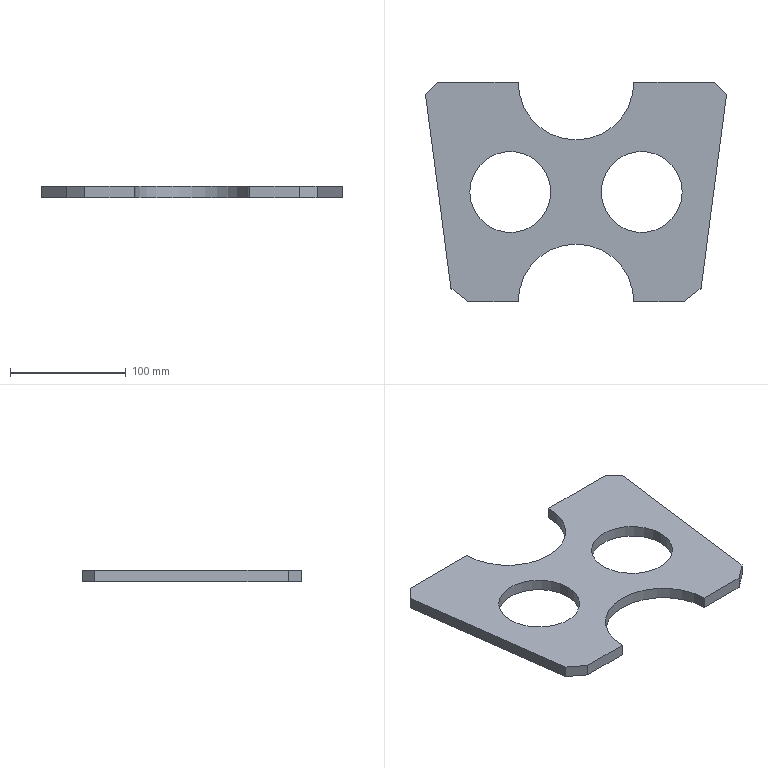Part | SolidWorks | features Extrusion 1 | 1 solid | 18 faces | box 260.209 x 190 x 10 mm | volume 293760 mm3 | plane 12 | cylinder 6 | commonest cylinder face diameters 70 x4 100 x2
STEP:
#1=CARTESIAN_POINT('',(-91.75,0.,10.));
#2=VERTEX_POINT('',#1);
#3=CARTESIAN_POINT('',(-21.75,0.,10.));
#4=VERTEX_POINT('',#3);
#5=CARTESIAN_POINT('',(-56.75,0.,10.));
#6=DIRECTION('',(0.,0.,1.));
#7=DIRECTION('',(-1.,0.,0.));
#8=AXIS2_PLACEMENT_3D('',#5,#6,#7);
#9=CIRCLE('',#8,35.);
#10=EDGE_CURVE('',#2,#4,#9,.T.);
#11=ORIENTED_EDGE('',*,*,#10,.T.);
#12=CARTESIAN_POINT('',(-21.75,0.,0.));
#13=VERTEX_POINT('',#12);
#14=CARTESIAN_POINT('',(-21.75,0.,10.));
#15=DIRECTION('',(0.,0.,-1.));
#16=VECTOR('',#15,1000.);
#17=LINE('',#14,#16);
#18=EDGE_CURVE('',#4,#13,#17,.T.);
#19=ORIENTED_EDGE('',*,*,#18,.T.);
#20=CARTESIAN_POINT('',(-91.75,0.,0.));
#21=VERTEX_POINT('',#20);
#22=CARTESIAN_POINT('',(-56.75,0.,0.));
#23=DIRECTION('',(0.,0.,1.));
#24=DIRECTION('',(-1.,0.,0.));
#25=AXIS2_PLACEMENT_3D('',#22,#23,#24);
#26=CIRCLE('',#25,35.);
#27=EDGE_CURVE('',#21,#13,#26,.T.);
#28=ORIENTED_EDGE('',*,*,#27,.F.);
#29=CARTESIAN_POINT('',(-91.75,0.,10.));
#30=DIRECTION('',(0.,0.,-1.));
#31=VECTOR('',#30,1000.);
#32=LINE('',#29,#31);
#33=EDGE_CURVE('',#2,#21,#32,.T.);
#34=ORIENTED_EDGE('',*,*,#33,.F.);
#35=EDGE_LOOP('',(#11,#19,#28,#34));
#36=FACE_OUTER_BOUND('',#35,.T.);
#37=CARTESIAN_POINT('',(-56.75,0.,10.));
#38=DIRECTION('',(0.,0.,-1.));
#39=DIRECTION('',(-1.,0.,0.));
#40=AXIS2_PLACEMENT_3D('',#37,#38,#39);
#41=CYLINDRICAL_SURFACE('',#40,35.);
#42=ADVANCED_FACE('',(#36),#41,.F.);
#43=CARTESIAN_POINT('',(21.75,0.,10.));
#44=VERTEX_POINT('',#43);
#45=CARTESIAN_POINT('',(91.75,0.,10.));
#46=VERTEX_POINT('',#45);
#47=CARTESIAN_POINT('',(56.75,0.,10.));
#48=DIRECTION('',(0.,0.,1.));
#49=DIRECTION('',(1.,0.,0.));
#50=AXIS2_PLACEMENT_3D('',#47,#48,#49);
#51=CIRCLE('',#50,35.);
#52=EDGE_CURVE('',#44,#46,#51,.T.);
#53=ORIENTED_EDGE('',*,*,#52,.T.);
#54=CARTESIAN_POINT('',(91.75,0.,0.));
#55=VERTEX_POINT('',#54);
#56=CARTESIAN_POINT('',(91.75,0.,10.));
#57=DIRECTION('',(0.,0.,-1.));
#58=VECTOR('',#57,1000.);
#59=LINE('',#56,#58);
#60=EDGE_CURVE('',#46,#55,#59,.T.);
#61=ORIENTED_EDGE('',*,*,#60,.T.);
#62=CARTESIAN_POINT('',(21.75,0.,0.));
#63=VERTEX_POINT('',#62);
#64=CARTESIAN_POINT('',(56.75,0.,0.));
#65=DIRECTION('',(0.,0.,1.));
#66=DIRECTION('',(1.,0.,0.));
#67=AXIS2_PLACEMENT_3D('',#64,#65,#66);
#68=CIRCLE('',#67,35.);
#69=EDGE_CURVE('',#63,#55,#68,.T.);
#70=ORIENTED_EDGE('',*,*,#69,.F.);
#71=CARTESIAN_POINT('',(21.75,0.,10.));
#72=DIRECTION('',(0.,0.,-1.));
#73=VECTOR('',#72,1000.);
#74=LINE('',#71,#73);
#75=EDGE_CURVE('',#44,#63,#74,.T.);
#76=ORIENTED_EDGE('',*,*,#75,.F.);
#77=EDGE_LOOP('',(#53,#61,#70,#76));
#78=FACE_OUTER_BOUND('',#77,.T.);
#79=CARTESIAN_POINT('',(56.75,0.,10.));
#80=DIRECTION('',(0.,0.,-1.));
#81=DIRECTION('',(-1.,0.,0.));
#82=AXIS2_PLACEMENT_3D('',#79,#80,#81);
#83=CYLINDRICAL_SURFACE('',#82,35.);
#84=ADVANCED_FACE('',(#78),#83,.F.);
#85=ORIENTED_EDGE('',*,*,#52,.F.);
#86=CARTESIAN_POINT('',(56.75,0.,10.));
#87=DIRECTION('',(0.,0.,1.));
#88=DIRECTION('',(1.,0.,0.));
#89=AXIS2_PLACEMENT_3D('',#86,#87,#88);
#90=CIRCLE('',#89,35.);
#91=EDGE_CURVE('',#46,#44,#90,.T.);
#92=ORIENTED_EDGE('',*,*,#91,.F.);
#93=EDGE_LOOP('',(#85,#92));
#94=FACE_BOUND('',#93,.T.);
#95=CARTESIAN_POINT('',(92.563,-95.,10.));
#96=VERTEX_POINT('',#95);
#97=CARTESIAN_POINT('',(108.065,-83.103,10.));
#98=VERTEX_POINT('',#97);
#99=CARTESIAN_POINT('',(108.065,-83.103,10.));
#100=DIRECTION('',(0.7933,0.6088,0.));
#101=VECTOR('',#100,1000.);
#102=LINE('',#99,#101);
#103=EDGE_CURVE('',#96,#98,#102,.T.);
#104=ORIENTED_EDGE('',*,*,#103,.T.);
#105=CARTESIAN_POINT('',(130.105,84.395,10.));
#106=VERTEX_POINT('',#105);
#107=CARTESIAN_POINT('',(130.105,84.395,10.));
#108=DIRECTION('',(0.1305,0.9915,0.));
#109=VECTOR('',#108,1000.);
#110=LINE('',#107,#109);
#111=EDGE_CURVE('',#98,#106,#110,.T.);
#112=ORIENTED_EDGE('',*,*,#111,.T.);
#113=CARTESIAN_POINT('',(119.5,95.,10.));
#114=VERTEX_POINT('',#113);
#115=CARTESIAN_POINT('',(119.5,95.,10.));
#116=DIRECTION('',(-0.7071,0.7071,0.));
#117=VECTOR('',#116,1000.);
#118=LINE('',#115,#117);
#119=EDGE_CURVE('',#106,#114,#118,.T.);
#120=ORIENTED_EDGE('',*,*,#119,.T.);
#121=CARTESIAN_POINT('',(50.,95.,10.));
#122=VERTEX_POINT('',#121);
#123=CARTESIAN_POINT('',(50.,95.,10.));
#124=DIRECTION('',(-1.,0.,0.));
#125=VECTOR('',#124,1000.);
#126=LINE('',#123,#125);
#127=EDGE_CURVE('',#114,#122,#126,.T.);
#128=ORIENTED_EDGE('',*,*,#127,.T.);
#129=CARTESIAN_POINT('',(-50.,95.,10.));
#130=VERTEX_POINT('',#129);
#131=CARTESIAN_POINT('',(0.,95.,10.));
#132=DIRECTION('',(0.,0.,-1.));
#133=DIRECTION('',(1.,0.,0.));
#134=AXIS2_PLACEMENT_3D('',#131,#132,#133);
#135=CIRCLE('',#134,50.);
#136=EDGE_CURVE('',#122,#130,#135,.T.);
#137=ORIENTED_EDGE('',*,*,#136,.T.);
#138=CARTESIAN_POINT('',(-119.5,95.,10.));
#139=VERTEX_POINT('',#138);
#140=CARTESIAN_POINT('',(-50.,95.,10.));
#141=DIRECTION('',(-1.,0.,0.));
#142=VECTOR('',#141,1000.);
#143=LINE('',#140,#142);
#144=EDGE_CURVE('',#130,#139,#143,.T.);
#145=ORIENTED_EDGE('',*,*,#144,.T.);
#146=CARTESIAN_POINT('',(-130.105,84.395,10.));
#147=VERTEX_POINT('',#146);
#148=CARTESIAN_POINT('',(-119.5,95.,10.));
#149=DIRECTION('',(-0.7071,-0.7071,0.));
#150=VECTOR('',#149,1000.);
#151=LINE('',#148,#150);
#152=EDGE_CURVE('',#139,#147,#151,.T.);
#153=ORIENTED_EDGE('',*,*,#152,.T.);
#154=CARTESIAN_POINT('',(-108.065,-83.103,10.));
#155=VERTEX_POINT('',#154);
#156=CARTESIAN_POINT('',(-130.105,84.395,10.));
#157=DIRECTION('',(0.1305,-0.9915,0.));
#158=VECTOR('',#157,1000.);
#159=LINE('',#156,#158);
#160=EDGE_CURVE('',#147,#155,#159,.T.);
#161=ORIENTED_EDGE('',*,*,#160,.T.);
#162=CARTESIAN_POINT('',(-92.563,-95.,10.));
#163=VERTEX_POINT('',#162);
#164=CARTESIAN_POINT('',(-108.065,-83.103,10.));
#165=DIRECTION('',(0.7933,-0.6088,0.));
#166=VECTOR('',#165,1000.);
#167=LINE('',#164,#166);
#168=EDGE_CURVE('',#155,#163,#167,.T.);
#169=ORIENTED_EDGE('',*,*,#168,.T.);
#170=CARTESIAN_POINT('',(-50.,-95.,10.));
#171=VERTEX_POINT('',#170);
#172=CARTESIAN_POINT('',(-50.,-95.,10.));
#173=DIRECTION('',(1.,0.,0.));
#174=VECTOR('',#173,1000.);
#175=LINE('',#172,#174);
#176=EDGE_CURVE('',#163,#171,#175,.T.);
#177=ORIENTED_EDGE('',*,*,#176,.T.);
#178=CARTESIAN_POINT('',(50.,-95.,10.));
#179=VERTEX_POINT('',#178);
#180=CARTESIAN_POINT('',(0.,-95.,10.));
#181=DIRECTION('',(0.,0.,-1.));
#182=DIRECTION('',(1.,0.,0.));
#183=AXIS2_PLACEMENT_3D('',#180,#181,#182);
#184=CIRCLE('',#183,50.);
#185=EDGE_CURVE('',#171,#179,#184,.T.);
#186=ORIENTED_EDGE('',*,*,#185,.T.);
#187=CARTESIAN_POINT('',(50.,-95.,10.));
#188=DIRECTION('',(1.,0.,0.));
#189=VECTOR('',#188,1000.);
#190=LINE('',#187,#189);
#191=EDGE_CURVE('',#179,#96,#190,.T.);
#192=ORIENTED_EDGE('',*,*,#191,.T.);
#193=EDGE_LOOP('',(#104,#112,#120,#128,#137,#145,#153,#161,#169,#177,#186,#192));
#194=FACE_OUTER_BOUND('',#193,.T.);
#195=ORIENTED_EDGE('',*,*,#10,.F.);
#196=CARTESIAN_POINT('',(-56.75,0.,10.));
#197=DIRECTION('',(0.,0.,1.));
#198=DIRECTION('',(-1.,0.,0.));
#199=AXIS2_PLACEMENT_3D('',#196,#197,#198);
#200=CIRCLE('',#199,35.);
#201=EDGE_CURVE('',#4,#2,#200,.T.);
#202=ORIENTED_EDGE('',*,*,#201,.F.);
#203=EDGE_LOOP('',(#195,#202));
#204=FACE_BOUND('',#203,.T.);
#205=CARTESIAN_POINT('',(0.,-95.,10.));
#206=DIRECTION('',(0.,0.,1.));
#207=DIRECTION('',(1.,0.,0.));
#208=AXIS2_PLACEMENT_3D('',#205,#206,#207);
#209=PLANE('',#208);
#210=ADVANCED_FACE('',(#94,#194,#204),#209,.T.);
#211=ORIENTED_EDGE('',*,*,#69,.T.);
#212=CARTESIAN_POINT('',(56.75,0.,0.));
#213=DIRECTION('',(0.,0.,1.));
#214=DIRECTION('',(1.,0.,0.));
#215=AXIS2_PLACEMENT_3D('',#212,#213,#214);
#216=CIRCLE('',#215,35.);
#217=EDGE_CURVE('',#55,#63,#216,.T.);
#218=ORIENTED_EDGE('',*,*,#217,.T.);
#219=EDGE_LOOP('',(#211,#218));
#220=FACE_BOUND('',#219,.T.);
#221=CARTESIAN_POINT('',(92.563,-95.,0.));
#222=VERTEX_POINT('',#221);
#223=CARTESIAN_POINT('',(108.065,-83.103,0.));
#224=VERTEX_POINT('',#223);
#225=CARTESIAN_POINT('',(108.065,-83.103,0.));
#226=DIRECTION('',(0.7933,0.6088,0.));
#227=VECTOR('',#226,1000.);
#228=LINE('',#225,#227);
#229=EDGE_CURVE('',#222,#224,#228,.T.);
#230=ORIENTED_EDGE('',*,*,#229,.F.);
#231=CARTESIAN_POINT('',(50.,-95.,0.));
#232=VERTEX_POINT('',#231);
#233=CARTESIAN_POINT('',(50.,-95.,0.));
#234=DIRECTION('',(1.,0.,0.));
#235=VECTOR('',#234,1000.);
#236=LINE('',#233,#235);
#237=EDGE_CURVE('',#232,#222,#236,.T.);
#238=ORIENTED_EDGE('',*,*,#237,.F.);
#239=CARTESIAN_POINT('',(-50.,-95.,0.));
#240=VERTEX_POINT('',#239);
#241=CARTESIAN_POINT('',(0.,-95.,0.));
#242=DIRECTION('',(0.,0.,-1.));
#243=DIRECTION('',(1.,0.,0.));
#244=AXIS2_PLACEMENT_3D('',#241,#242,#243);
#245=CIRCLE('',#244,50.);
#246=EDGE_CURVE('',#240,#232,#245,.T.);
#247=ORIENTED_EDGE('',*,*,#246,.F.);
#248=CARTESIAN_POINT('',(-92.563,-95.,0.));
#249=VERTEX_POINT('',#248);
#250=CARTESIAN_POINT('',(-50.,-95.,0.));
#251=DIRECTION('',(1.,0.,0.));
#252=VECTOR('',#251,1000.);
#253=LINE('',#250,#252);
#254=EDGE_CURVE('',#249,#240,#253,.T.);
#255=ORIENTED_EDGE('',*,*,#254,.F.);
#256=CARTESIAN_POINT('',(-108.065,-83.103,0.));
#257=VERTEX_POINT('',#256);
#258=CARTESIAN_POINT('',(-108.065,-83.103,0.));
#259=DIRECTION('',(0.7933,-0.6088,0.));
#260=VECTOR('',#259,1000.);
#261=LINE('',#258,#260);
#262=EDGE_CURVE('',#257,#249,#261,.T.);
#263=ORIENTED_EDGE('',*,*,#262,.F.);
#264=CARTESIAN_POINT('',(-130.105,84.395,0.));
#265=VERTEX_POINT('',#264);
#266=CARTESIAN_POINT('',(-130.105,84.395,0.));
#267=DIRECTION('',(0.1305,-0.9915,0.));
#268=VECTOR('',#267,1000.);
#269=LINE('',#266,#268);
#270=EDGE_CURVE('',#265,#257,#269,.T.);
#271=ORIENTED_EDGE('',*,*,#270,.F.);
#272=CARTESIAN_POINT('',(-119.5,95.,0.));
#273=VERTEX_POINT('',#272);
#274=CARTESIAN_POINT('',(-119.5,95.,0.));
#275=DIRECTION('',(-0.7071,-0.7071,0.));
#276=VECTOR('',#275,1000.);
#277=LINE('',#274,#276);
#278=EDGE_CURVE('',#273,#265,#277,.T.);
#279=ORIENTED_EDGE('',*,*,#278,.F.);
#280=CARTESIAN_POINT('',(-50.,95.,0.));
#281=VERTEX_POINT('',#280);
#282=CARTESIAN_POINT('',(-50.,95.,0.));
#283=DIRECTION('',(-1.,0.,0.));
#284=VECTOR('',#283,1000.);
#285=LINE('',#282,#284);
#286=EDGE_CURVE('',#281,#273,#285,.T.);
#287=ORIENTED_EDGE('',*,*,#286,.F.);
#288=CARTESIAN_POINT('',(50.,95.,0.));
#289=VERTEX_POINT('',#288);
#290=CARTESIAN_POINT('',(0.,95.,0.));
#291=DIRECTION('',(0.,0.,-1.));
#292=DIRECTION('',(1.,0.,0.));
#293=AXIS2_PLACEMENT_3D('',#290,#291,#292);
#294=CIRCLE('',#293,50.);
#295=EDGE_CURVE('',#289,#281,#294,.T.);
#296=ORIENTED_EDGE('',*,*,#295,.F.);
#297=CARTESIAN_POINT('',(119.5,95.,0.));
#298=VERTEX_POINT('',#297);
#299=CARTESIAN_POINT('',(50.,95.,0.));
#300=DIRECTION('',(-1.,0.,0.));
#301=VECTOR('',#300,1000.);
#302=LINE('',#299,#301);
#303=EDGE_CURVE('',#298,#289,#302,.T.);
#304=ORIENTED_EDGE('',*,*,#303,.F.);
#305=CARTESIAN_POINT('',(130.105,84.395,0.));
#306=VERTEX_POINT('',#305);
#307=CARTESIAN_POINT('',(119.5,95.,0.));
#308=DIRECTION('',(-0.7071,0.7071,0.));
#309=VECTOR('',#308,1000.);
#310=LINE('',#307,#309);
#311=EDGE_CURVE('',#306,#298,#310,.T.);
#312=ORIENTED_EDGE('',*,*,#311,.F.);
#313=CARTESIAN_POINT('',(130.105,84.395,0.));
#314=DIRECTION('',(0.1305,0.9915,0.));
#315=VECTOR('',#314,1000.);
#316=LINE('',#313,#315);
#317=EDGE_CURVE('',#224,#306,#316,.T.);
#318=ORIENTED_EDGE('',*,*,#317,.F.);
#319=EDGE_LOOP('',(#230,#238,#247,#255,#263,#271,#279,#287,#296,#304,#312,#318));
#320=FACE_OUTER_BOUND('',#319,.T.);
#321=ORIENTED_EDGE('',*,*,#27,.T.);
#322=CARTESIAN_POINT('',(-56.75,0.,0.));
#323=DIRECTION('',(0.,0.,1.));
#324=DIRECTION('',(-1.,0.,0.));
#325=AXIS2_PLACEMENT_3D('',#322,#323,#324);
#326=CIRCLE('',#325,35.);
#327=EDGE_CURVE('',#13,#21,#326,.T.);
#328=ORIENTED_EDGE('',*,*,#327,.T.);
#329=EDGE_LOOP('',(#321,#328));
#330=FACE_BOUND('',#329,.T.);
#331=CARTESIAN_POINT('',(0.,-95.,0.));
#332=DIRECTION('',(0.,0.,1.));
#333=DIRECTION('',(1.,0.,0.));
#334=AXIS2_PLACEMENT_3D('',#331,#332,#333);
#335=PLANE('',#334);
#336=ADVANCED_FACE('',(#220,#320,#330),#335,.F.);
#337=ORIENTED_EDGE('',*,*,#229,.T.);
#338=CARTESIAN_POINT('',(108.065,-83.103,10.));
#339=DIRECTION('',(0.,0.,-1.));
#340=VECTOR('',#339,1000.);
#341=LINE('',#338,#340);
#342=EDGE_CURVE('',#98,#224,#341,.T.);
#343=ORIENTED_EDGE('',*,*,#342,.F.);
#344=ORIENTED_EDGE('',*,*,#103,.F.);
#345=CARTESIAN_POINT('',(92.563,-95.,10.));
#346=DIRECTION('',(0.,0.,-1.));
#347=VECTOR('',#346,1000.);
#348=LINE('',#345,#347);
#349=EDGE_CURVE('',#96,#222,#348,.T.);
#350=ORIENTED_EDGE('',*,*,#349,.T.);
#351=EDGE_LOOP('',(#337,#343,#344,#350));
#352=FACE_OUTER_BOUND('',#351,.T.);
#353=CARTESIAN_POINT('',(108.065,-83.103,10.));
#354=DIRECTION('',(-0.6088,0.7933,0.));
#355=DIRECTION('',(-0.7933,-0.6088,0.));
#356=AXIS2_PLACEMENT_3D('',#353,#354,#355);
#357=PLANE('',#356);
#358=ADVANCED_FACE('',(#352),#357,.F.);
#359=ORIENTED_EDGE('',*,*,#317,.T.);
#360=CARTESIAN_POINT('',(130.105,84.395,10.));
#361=DIRECTION('',(0.,0.,-1.));
#362=VECTOR('',#361,1000.);
#363=LINE('',#360,#362);
#364=EDGE_CURVE('',#106,#306,#363,.T.);
#365=ORIENTED_EDGE('',*,*,#364,.F.);
#366=ORIENTED_EDGE('',*,*,#111,.F.);
#367=ORIENTED_EDGE('',*,*,#342,.T.);
#368=EDGE_LOOP('',(#359,#365,#366,#367));
#369=FACE_OUTER_BOUND('',#368,.T.);
#370=CARTESIAN_POINT('',(130.105,84.395,10.));
#371=DIRECTION('',(-0.9915,0.1305,0.));
#372=DIRECTION('',(-0.1305,-0.9915,0.));
#373=AXIS2_PLACEMENT_3D('',#370,#371,#372);
#374=PLANE('',#373);
#375=ADVANCED_FACE('',(#369),#374,.F.);
#376=ORIENTED_EDGE('',*,*,#311,.T.);
#377=CARTESIAN_POINT('',(119.5,95.,10.));
#378=DIRECTION('',(0.,0.,-1.));
#379=VECTOR('',#378,1000.);
#380=LINE('',#377,#379);
#381=EDGE_CURVE('',#114,#298,#380,.T.);
#382=ORIENTED_EDGE('',*,*,#381,.F.);
#383=ORIENTED_EDGE('',*,*,#119,.F.);
#384=ORIENTED_EDGE('',*,*,#364,.T.);
#385=EDGE_LOOP('',(#376,#382,#383,#384));
#386=FACE_OUTER_BOUND('',#385,.T.);
#387=CARTESIAN_POINT('',(119.5,95.,10.));
#388=DIRECTION('',(-0.7071,-0.7071,0.));
#389=DIRECTION('',(0.7071,-0.7071,0.));
#390=AXIS2_PLACEMENT_3D('',#387,#388,#389);
#391=PLANE('',#390);
#392=ADVANCED_FACE('',(#386),#391,.F.);
#393=ORIENTED_EDGE('',*,*,#303,.T.);
#394=CARTESIAN_POINT('',(50.,95.,10.));
#395=DIRECTION('',(0.,0.,-1.));
#396=VECTOR('',#395,1000.);
#397=LINE('',#394,#396);
#398=EDGE_CURVE('',#122,#289,#397,.T.);
#399=ORIENTED_EDGE('',*,*,#398,.F.);
#400=ORIENTED_EDGE('',*,*,#127,.F.);
#401=ORIENTED_EDGE('',*,*,#381,.T.);
#402=EDGE_LOOP('',(#393,#399,#400,#401));
#403=FACE_OUTER_BOUND('',#402,.T.);
#404=CARTESIAN_POINT('',(50.,95.,10.));
#405=DIRECTION('',(0.,-1.,0.));
#406=DIRECTION('',(0.,0.,-1.));
#407=AXIS2_PLACEMENT_3D('',#404,#405,#406);
#408=PLANE('',#407);
#409=ADVANCED_FACE('',(#403),#408,.F.);
#410=ORIENTED_EDGE('',*,*,#295,.T.);
#411=CARTESIAN_POINT('',(-50.,95.,10.));
#412=DIRECTION('',(0.,0.,-1.));
#413=VECTOR('',#412,1000.);
#414=LINE('',#411,#413);
#415=EDGE_CURVE('',#130,#281,#414,.T.);
#416=ORIENTED_EDGE('',*,*,#415,.F.);
#417=ORIENTED_EDGE('',*,*,#136,.F.);
#418=ORIENTED_EDGE('',*,*,#398,.T.);
#419=EDGE_LOOP('',(#410,#416,#417,#418));
#420=FACE_OUTER_BOUND('',#419,.T.);
#421=CARTESIAN_POINT('',(0.,95.,10.));
#422=DIRECTION('',(0.,0.,-1.));
#423=DIRECTION('',(-1.,0.,0.));
#424=AXIS2_PLACEMENT_3D('',#421,#422,#423);
#425=CYLINDRICAL_SURFACE('',#424,50.);
#426=ADVANCED_FACE('',(#420),#425,.F.);
#427=ORIENTED_EDGE('',*,*,#286,.T.);
#428=CARTESIAN_POINT('',(-119.5,95.,10.));
#429=DIRECTION('',(0.,0.,-1.));
#430=VECTOR('',#429,1000.);
#431=LINE('',#428,#430);
#432=EDGE_CURVE('',#139,#273,#431,.T.);
#433=ORIENTED_EDGE('',*,*,#432,.F.);
#434=ORIENTED_EDGE('',*,*,#144,.F.);
#435=ORIENTED_EDGE('',*,*,#415,.T.);
#436=EDGE_LOOP('',(#427,#433,#434,#435));
#437=FACE_OUTER_BOUND('',#436,.T.);
#438=CARTESIAN_POINT('',(-50.,95.,10.));
#439=DIRECTION('',(0.,-1.,0.));
#440=DIRECTION('',(0.,0.,-1.));
#441=AXIS2_PLACEMENT_3D('',#438,#439,#440);
#442=PLANE('',#441);
#443=ADVANCED_FACE('',(#437),#442,.F.);
#444=ORIENTED_EDGE('',*,*,#278,.T.);
#445=CARTESIAN_POINT('',(-130.105,84.395,10.));
#446=DIRECTION('',(0.,0.,-1.));
#447=VECTOR('',#446,1000.);
#448=LINE('',#445,#447);
#449=EDGE_CURVE('',#147,#265,#448,.T.);
#450=ORIENTED_EDGE('',*,*,#449,.F.);
#451=ORIENTED_EDGE('',*,*,#152,.F.);
#452=ORIENTED_EDGE('',*,*,#432,.T.);
#453=EDGE_LOOP('',(#444,#450,#451,#452));
#454=FACE_OUTER_BOUND('',#453,.T.);
#455=CARTESIAN_POINT('',(-119.5,95.,10.));
#456=DIRECTION('',(0.7071,-0.7071,0.));
#457=DIRECTION('',(0.7071,0.7071,0.));
#458=AXIS2_PLACEMENT_3D('',#455,#456,#457);
#459=PLANE('',#458);
#460=ADVANCED_FACE('',(#454),#459,.F.);
#461=ORIENTED_EDGE('',*,*,#270,.T.);
#462=CARTESIAN_POINT('',(-108.065,-83.103,10.));
#463=DIRECTION('',(0.,0.,-1.));
#464=VECTOR('',#463,1000.);
#465=LINE('',#462,#464);
#466=EDGE_CURVE('',#155,#257,#465,.T.);
#467=ORIENTED_EDGE('',*,*,#466,.F.);
#468=ORIENTED_EDGE('',*,*,#160,.F.);
#469=ORIENTED_EDGE('',*,*,#449,.T.);
#470=EDGE_LOOP('',(#461,#467,#468,#469));
#471=FACE_OUTER_BOUND('',#470,.T.);
#472=CARTESIAN_POINT('',(-130.105,84.395,10.));
#473=DIRECTION('',(0.9915,0.1305,0.));
#474=DIRECTION('',(-0.1305,0.9915,0.));
#475=AXIS2_PLACEMENT_3D('',#472,#473,#474);
#476=PLANE('',#475);
#477=ADVANCED_FACE('',(#471),#476,.F.);
#478=ORIENTED_EDGE('',*,*,#262,.T.);
#479=CARTESIAN_POINT('',(-92.563,-95.,10.));
#480=DIRECTION('',(0.,0.,-1.));
#481=VECTOR('',#480,1000.);
#482=LINE('',#479,#481);
#483=EDGE_CURVE('',#163,#249,#482,.T.);
#484=ORIENTED_EDGE('',*,*,#483,.F.);
#485=ORIENTED_EDGE('',*,*,#168,.F.);
#486=ORIENTED_EDGE('',*,*,#466,.T.);
#487=EDGE_LOOP('',(#478,#484,#485,#486));
#488=FACE_OUTER_BOUND('',#487,.T.);
#489=CARTESIAN_POINT('',(-108.065,-83.103,10.));
#490=DIRECTION('',(0.6088,0.7933,0.));
#491=DIRECTION('',(-0.7933,0.6088,0.));
#492=AXIS2_PLACEMENT_3D('',#489,#490,#491);
#493=PLANE('',#492);
#494=ADVANCED_FACE('',(#488),#493,.F.);
#495=ORIENTED_EDGE('',*,*,#254,.T.);
#496=CARTESIAN_POINT('',(-50.,-95.,10.));
#497=DIRECTION('',(0.,0.,-1.));
#498=VECTOR('',#497,1000.);
#499=LINE('',#496,#498);
#500=EDGE_CURVE('',#171,#240,#499,.T.);
#501=ORIENTED_EDGE('',*,*,#500,.F.);
#502=ORIENTED_EDGE('',*,*,#176,.F.);
#503=ORIENTED_EDGE('',*,*,#483,.T.);
#504=EDGE_LOOP('',(#495,#501,#502,#503));
#505=FACE_OUTER_BOUND('',#504,.T.);
#506=CARTESIAN_POINT('',(-50.,-95.,10.));
#507=DIRECTION('',(0.,1.,0.));
#508=DIRECTION('',(-1.,0.,0.));
#509=AXIS2_PLACEMENT_3D('',#506,#507,#508);
#510=PLANE('',#509);
#511=ADVANCED_FACE('',(#505),#510,.F.);
#512=ORIENTED_EDGE('',*,*,#246,.T.);
#513=CARTESIAN_POINT('',(50.,-95.,10.));
#514=DIRECTION('',(0.,0.,-1.));
#515=VECTOR('',#514,1000.);
#516=LINE('',#513,#515);
#517=EDGE_CURVE('',#179,#232,#516,.T.);
#518=ORIENTED_EDGE('',*,*,#517,.F.);
#519=ORIENTED_EDGE('',*,*,#185,.F.);
#520=ORIENTED_EDGE('',*,*,#500,.T.);
#521=EDGE_LOOP('',(#512,#518,#519,#520));
#522=FACE_OUTER_BOUND('',#521,.T.);
#523=CARTESIAN_POINT('',(0.,-95.,10.));
#524=DIRECTION('',(0.,0.,-1.));
#525=DIRECTION('',(-1.,0.,0.));
#526=AXIS2_PLACEMENT_3D('',#523,#524,#525);
#527=CYLINDRICAL_SURFACE('',#526,50.);
#528=ADVANCED_FACE('',(#522),#527,.F.);
#529=ORIENTED_EDGE('',*,*,#237,.T.);
#530=ORIENTED_EDGE('',*,*,#349,.F.);
#531=ORIENTED_EDGE('',*,*,#191,.F.);
#532=ORIENTED_EDGE('',*,*,#517,.T.);
#533=EDGE_LOOP('',(#529,#530,#531,#532));
#534=FACE_OUTER_BOUND('',#533,.T.);
#535=CARTESIAN_POINT('',(50.,-95.,10.));
#536=DIRECTION('',(0.,1.,0.));
#537=DIRECTION('',(-1.,0.,0.));
#538=AXIS2_PLACEMENT_3D('',#535,#536,#537);
#539=PLANE('',#538);
#540=ADVANCED_FACE('',(#534),#539,.F.);
#541=ORIENTED_EDGE('',*,*,#60,.F.);
#542=ORIENTED_EDGE('',*,*,#91,.T.);
#543=ORIENTED_EDGE('',*,*,#75,.T.);
#544=ORIENTED_EDGE('',*,*,#217,.F.);
#545=EDGE_LOOP('',(#541,#542,#543,#544));
#546=FACE_OUTER_BOUND('',#545,.T.);
#547=CARTESIAN_POINT('',(56.75,0.,10.));
#548=DIRECTION('',(0.,0.,-1.));
#549=DIRECTION('',(-1.,0.,0.));
#550=AXIS2_PLACEMENT_3D('',#547,#548,#549);
#551=CYLINDRICAL_SURFACE('',#550,35.);
#552=ADVANCED_FACE('',(#546),#551,.F.);
#553=ORIENTED_EDGE('',*,*,#18,.F.);
#554=ORIENTED_EDGE('',*,*,#201,.T.);
#555=ORIENTED_EDGE('',*,*,#33,.T.);
#556=ORIENTED_EDGE('',*,*,#327,.F.);
#557=EDGE_LOOP('',(#553,#554,#555,#556));
#558=FACE_OUTER_BOUND('',#557,.T.);
#559=CARTESIAN_POINT('',(-56.75,0.,10.));
#560=DIRECTION('',(0.,0.,-1.));
#561=DIRECTION('',(-1.,0.,0.));
#562=AXIS2_PLACEMENT_3D('',#559,#560,#561);
#563=CYLINDRICAL_SURFACE('',#562,35.);
#564=ADVANCED_FACE('',(#558),#563,.F.);
#565=CLOSED_SHELL('',(#42,#84,#210,#336,#358,#375,#392,#409,#426,#443,#460,#477,#494,#511,#528,#540,#552,#564));
#566=MANIFOLD_SOLID_BREP('',#565);
#567=CARTESIAN_POINT('',(0.,0.,0.));
#568=DIRECTION('',(0.,0.,1.));
#569=DIRECTION('',(1.,0.,0.));
#570=AXIS2_PLACEMENT_3D('',#567,#568,#569);
#571=(LENGTH_UNIT()NAMED_UNIT(*)SI_UNIT(.MILLI.,.METRE.));
#572=UNCERTAINTY_MEASURE_WITH_UNIT(LENGTH_MEASURE(0.00001),#571,'','');
#573=(NAMED_UNIT(*)PLANE_ANGLE_UNIT()SI_UNIT($,.RADIAN.));
#574=(NAMED_UNIT(*)SI_UNIT($,.STERADIAN.)SOLID_ANGLE_UNIT());
#575=(GEOMETRIC_REPRESENTATION_CONTEXT(3)GLOBAL_UNCERTAINTY_ASSIGNED_CONTEXT((#572))GLOBAL_UNIT_ASSIGNED_CONTEXT((#571,#573,#574))REPRESENTATION_CONTEXT('',''));
#576=ADVANCED_BREP_SHAPE_REPRESENTATION('',(#566,#570),#575);